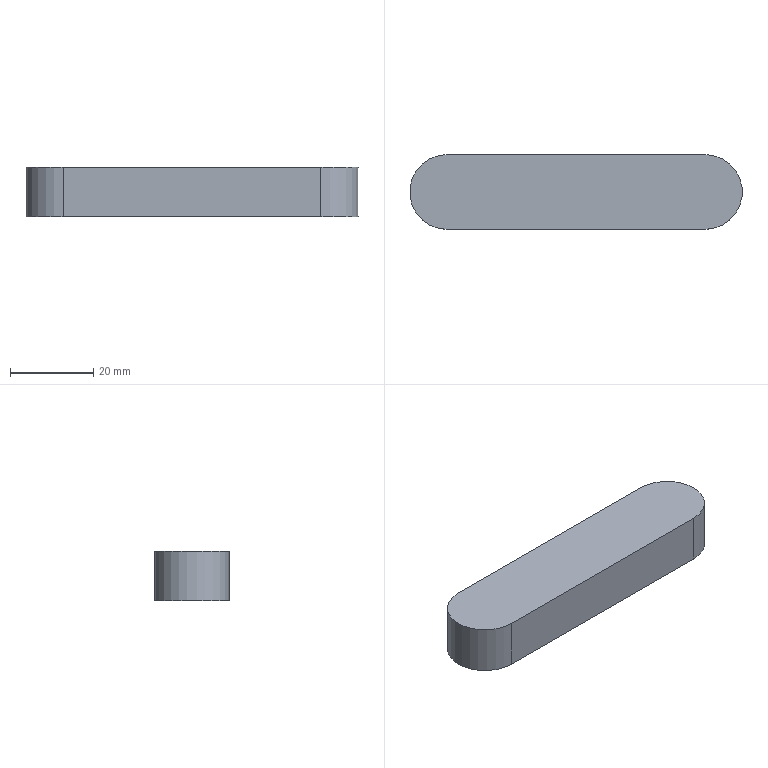Part | NX | features DATUM_CSYS 2, EXTRUDE 1, SKETCH 1 | 1 solid | 6 faces | box 80 x 18 x 12 mm | volume 16446 mm3 | plane 4 | cylinder 2 | commonest cylinder face diameters 18 x2
STEP:
#1=CARTESIAN_POINT('',(31.,-9.,0.));
#2=VERTEX_POINT('',#1);
#3=CARTESIAN_POINT('',(31.,9.,0.));
#4=VERTEX_POINT('',#3);
#5=CARTESIAN_POINT('',(31.,0.,0.));
#6=DIRECTION('',(0.,0.,1.));
#7=DIRECTION('',(-1.,0.,0.));
#8=AXIS2_PLACEMENT_3D('',#5,#6,#7);
#9=CIRCLE('',#8,9.);
#10=EDGE_CURVE('',#2,#4,#9,.T.);
#11=ORIENTED_EDGE('',*,*,#10,.T.);
#12=CARTESIAN_POINT('',(31.,9.,12.));
#13=VERTEX_POINT('',#12);
#14=CARTESIAN_POINT('',(31.,9.,12.));
#15=DIRECTION('',(0.,0.,-1.));
#16=VECTOR('',#15,1000.);
#17=LINE('',#14,#16);
#18=EDGE_CURVE('',#13,#4,#17,.T.);
#19=ORIENTED_EDGE('',*,*,#18,.F.);
#20=CARTESIAN_POINT('',(31.,-9.,12.));
#21=VERTEX_POINT('',#20);
#22=CARTESIAN_POINT('',(31.,0.,12.));
#23=DIRECTION('',(0.,0.,1.));
#24=DIRECTION('',(-1.,0.,0.));
#25=AXIS2_PLACEMENT_3D('',#22,#23,#24);
#26=CIRCLE('',#25,9.);
#27=EDGE_CURVE('',#21,#13,#26,.T.);
#28=ORIENTED_EDGE('',*,*,#27,.F.);
#29=CARTESIAN_POINT('',(31.,-9.,12.));
#30=DIRECTION('',(0.,0.,-1.));
#31=VECTOR('',#30,1000.);
#32=LINE('',#29,#31);
#33=EDGE_CURVE('',#21,#2,#32,.T.);
#34=ORIENTED_EDGE('',*,*,#33,.T.);
#35=EDGE_LOOP('',(#11,#19,#28,#34));
#36=FACE_BOUND('',#35,.T.);
#37=CARTESIAN_POINT('',(31.,0.,12.));
#38=DIRECTION('',(0.,0.,-1.));
#39=DIRECTION('',(-1.,0.,0.));
#40=AXIS2_PLACEMENT_3D('',#37,#38,#39);
#41=CYLINDRICAL_SURFACE('',#40,9.);
#42=ADVANCED_FACE('',(#36),#41,.T.);
#43=CARTESIAN_POINT('',(-31.,9.,0.));
#44=VERTEX_POINT('',#43);
#45=CARTESIAN_POINT('',(31.,9.,0.));
#46=DIRECTION('',(-1.,0.,0.));
#47=VECTOR('',#46,1000.);
#48=LINE('',#45,#47);
#49=EDGE_CURVE('',#4,#44,#48,.T.);
#50=ORIENTED_EDGE('',*,*,#49,.T.);
#51=CARTESIAN_POINT('',(-31.,9.,12.));
#52=VERTEX_POINT('',#51);
#53=CARTESIAN_POINT('',(-31.,9.,12.));
#54=DIRECTION('',(0.,0.,-1.));
#55=VECTOR('',#54,1000.);
#56=LINE('',#53,#55);
#57=EDGE_CURVE('',#52,#44,#56,.T.);
#58=ORIENTED_EDGE('',*,*,#57,.F.);
#59=CARTESIAN_POINT('',(31.,9.,12.));
#60=DIRECTION('',(-1.,0.,0.));
#61=VECTOR('',#60,1000.);
#62=LINE('',#59,#61);
#63=EDGE_CURVE('',#13,#52,#62,.T.);
#64=ORIENTED_EDGE('',*,*,#63,.F.);
#65=ORIENTED_EDGE('',*,*,#18,.T.);
#66=EDGE_LOOP('',(#50,#58,#64,#65));
#67=FACE_BOUND('',#66,.T.);
#68=CARTESIAN_POINT('',(31.,9.,12.));
#69=DIRECTION('',(0.,-1.,0.));
#70=DIRECTION('',(0.,0.,-1.));
#71=AXIS2_PLACEMENT_3D('',#68,#69,#70);
#72=PLANE('',#71);
#73=ADVANCED_FACE('',(#67),#72,.F.);
#74=CARTESIAN_POINT('',(-31.,-9.,0.));
#75=VERTEX_POINT('',#74);
#76=CARTESIAN_POINT('',(-31.,0.,0.));
#77=DIRECTION('',(0.,0.,1.));
#78=DIRECTION('',(1.,0.,0.));
#79=AXIS2_PLACEMENT_3D('',#76,#77,#78);
#80=CIRCLE('',#79,9.);
#81=EDGE_CURVE('',#44,#75,#80,.T.);
#82=ORIENTED_EDGE('',*,*,#81,.T.);
#83=CARTESIAN_POINT('',(-31.,-9.,12.));
#84=VERTEX_POINT('',#83);
#85=CARTESIAN_POINT('',(-31.,-9.,12.));
#86=DIRECTION('',(0.,0.,-1.));
#87=VECTOR('',#86,1000.);
#88=LINE('',#85,#87);
#89=EDGE_CURVE('',#84,#75,#88,.T.);
#90=ORIENTED_EDGE('',*,*,#89,.F.);
#91=CARTESIAN_POINT('',(-31.,0.,12.));
#92=DIRECTION('',(0.,0.,1.));
#93=DIRECTION('',(1.,0.,0.));
#94=AXIS2_PLACEMENT_3D('',#91,#92,#93);
#95=CIRCLE('',#94,9.);
#96=EDGE_CURVE('',#52,#84,#95,.T.);
#97=ORIENTED_EDGE('',*,*,#96,.F.);
#98=ORIENTED_EDGE('',*,*,#57,.T.);
#99=EDGE_LOOP('',(#82,#90,#97,#98));
#100=FACE_BOUND('',#99,.T.);
#101=CARTESIAN_POINT('',(-31.,0.,12.));
#102=DIRECTION('',(0.,0.,-1.));
#103=DIRECTION('',(-1.,0.,0.));
#104=AXIS2_PLACEMENT_3D('',#101,#102,#103);
#105=CYLINDRICAL_SURFACE('',#104,9.);
#106=ADVANCED_FACE('',(#100),#105,.T.);
#107=CARTESIAN_POINT('',(-31.,-9.,0.));
#108=DIRECTION('',(1.,0.,0.));
#109=VECTOR('',#108,1000.);
#110=LINE('',#107,#109);
#111=EDGE_CURVE('',#75,#2,#110,.T.);
#112=ORIENTED_EDGE('',*,*,#111,.T.);
#113=ORIENTED_EDGE('',*,*,#33,.F.);
#114=CARTESIAN_POINT('',(-31.,-9.,12.));
#115=DIRECTION('',(1.,0.,0.));
#116=VECTOR('',#115,1000.);
#117=LINE('',#114,#116);
#118=EDGE_CURVE('',#84,#21,#117,.T.);
#119=ORIENTED_EDGE('',*,*,#118,.F.);
#120=ORIENTED_EDGE('',*,*,#89,.T.);
#121=EDGE_LOOP('',(#112,#113,#119,#120));
#122=FACE_BOUND('',#121,.T.);
#123=CARTESIAN_POINT('',(-31.,-9.,12.));
#124=DIRECTION('',(0.,1.,0.));
#125=DIRECTION('',(0.,0.,1.));
#126=AXIS2_PLACEMENT_3D('',#123,#124,#125);
#127=PLANE('',#126);
#128=ADVANCED_FACE('',(#122),#127,.F.);
#129=ORIENTED_EDGE('',*,*,#27,.T.);
#130=ORIENTED_EDGE('',*,*,#63,.T.);
#131=ORIENTED_EDGE('',*,*,#96,.T.);
#132=ORIENTED_EDGE('',*,*,#118,.T.);
#133=EDGE_LOOP('',(#129,#130,#131,#132));
#134=FACE_BOUND('',#133,.T.);
#135=CARTESIAN_POINT('',(31.,0.,12.));
#136=DIRECTION('',(0.,0.,1.));
#137=DIRECTION('',(1.,0.,0.));
#138=AXIS2_PLACEMENT_3D('',#135,#136,#137);
#139=PLANE('',#138);
#140=ADVANCED_FACE('',(#134),#139,.T.);
#141=ORIENTED_EDGE('',*,*,#10,.F.);
#142=ORIENTED_EDGE('',*,*,#111,.F.);
#143=ORIENTED_EDGE('',*,*,#81,.F.);
#144=ORIENTED_EDGE('',*,*,#49,.F.);
#145=EDGE_LOOP('',(#141,#142,#143,#144));
#146=FACE_BOUND('',#145,.T.);
#147=CARTESIAN_POINT('',(31.,0.,0.));
#148=DIRECTION('',(0.,0.,1.));
#149=DIRECTION('',(1.,0.,0.));
#150=AXIS2_PLACEMENT_3D('',#147,#148,#149);
#151=PLANE('',#150);
#152=ADVANCED_FACE('',(#146),#151,.F.);
#153=CLOSED_SHELL('',(#42,#73,#106,#128,#140,#152));
#154=MANIFOLD_SOLID_BREP('',#153);
#155=(LENGTH_UNIT()NAMED_UNIT(*)SI_UNIT(.MILLI.,.METRE.));
#156=UNCERTAINTY_MEASURE_WITH_UNIT(LENGTH_MEASURE(0.00001),#155,'','');
#157=(NAMED_UNIT(*)PLANE_ANGLE_UNIT()SI_UNIT($,.RADIAN.));
#158=(NAMED_UNIT(*)SI_UNIT($,.STERADIAN.)SOLID_ANGLE_UNIT());
#159=(GEOMETRIC_REPRESENTATION_CONTEXT(3)GLOBAL_UNCERTAINTY_ASSIGNED_CONTEXT((#156))GLOBAL_UNIT_ASSIGNED_CONTEXT((#155,#157,#158))REPRESENTATION_CONTEXT('',''));
#160=ADVANCED_BREP_SHAPE_REPRESENTATION('',(#154),#159);